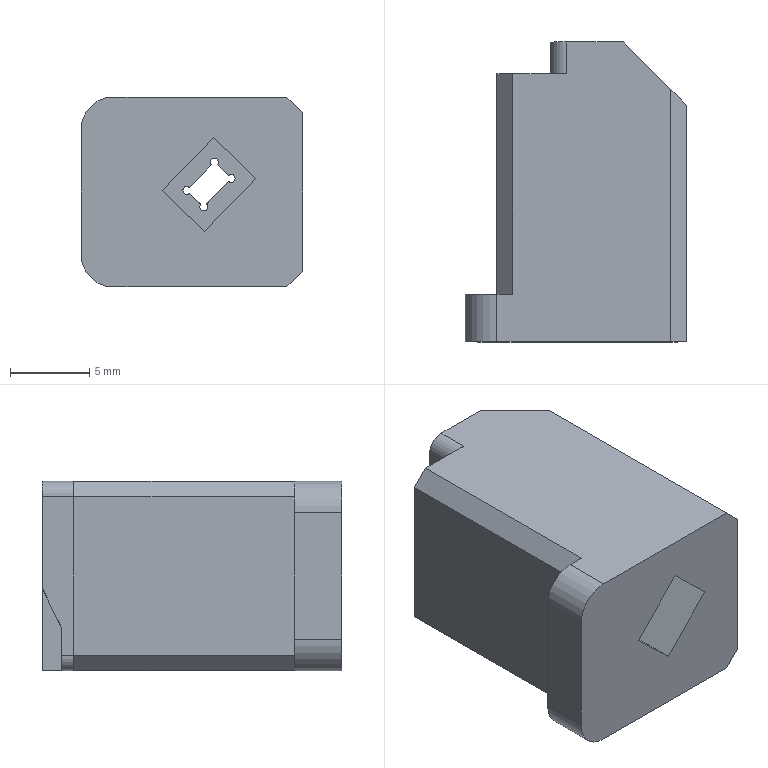Part | STEP file | 03-03 right cutter pad block | 1 solid | 46 faces | box 14 x 18.95 x 12 mm | volume 2331 mm3 | plane 29 | cylinder 17 | commonest cylinder face diameters 0.5 x9 0.6 x4 2 x2 4 x2
STEP:
#1=CARTESIAN_POINT('',(-2.2,16.95,-0.1351));
#2=VERTEX_POINT('',#1);
#3=CARTESIAN_POINT('',(-2.2,16.95,0.4649));
#4=VERTEX_POINT('',#3);
#5=CARTESIAN_POINT('',(-2.2,16.95,0.1649));
#6=DIRECTION('',(0.,1.,0.));
#7=DIRECTION('',(0.,0.,1.));
#8=AXIS2_PLACEMENT_3D('',#5,#6,#7);
#9=CIRCLE('',#8,0.3);
#10=EDGE_CURVE('',#2,#4,#9,.T.);
#11=ORIENTED_EDGE('',*,*,#10,.F.);
#12=CARTESIAN_POINT('',(-2.2,18.95,-0.1351));
#13=VERTEX_POINT('',#12);
#14=CARTESIAN_POINT('',(-2.2,16.95,-0.1351));
#15=DIRECTION('',(0.,1.,0.));
#16=VECTOR('',#15,1000.);
#17=LINE('',#14,#16);
#18=EDGE_CURVE('',#2,#13,#17,.T.);
#19=ORIENTED_EDGE('',*,*,#18,.T.);
#20=CARTESIAN_POINT('',(-2.2,18.95,0.4649));
#21=VERTEX_POINT('',#20);
#22=CARTESIAN_POINT('',(-2.2,18.95,0.1649));
#23=DIRECTION('',(0.,1.,0.));
#24=DIRECTION('',(0.,0.,1.));
#25=AXIS2_PLACEMENT_3D('',#22,#23,#24);
#26=CIRCLE('',#25,0.3);
#27=EDGE_CURVE('',#13,#21,#26,.T.);
#28=ORIENTED_EDGE('',*,*,#27,.T.);
#29=CARTESIAN_POINT('',(-2.2,16.95,0.4649));
#30=DIRECTION('',(0.,1.,0.));
#31=VECTOR('',#30,1000.);
#32=LINE('',#29,#31);
#33=EDGE_CURVE('',#4,#21,#32,.T.);
#34=ORIENTED_EDGE('',*,*,#33,.F.);
#35=EDGE_LOOP('',(#11,#19,#28,#34));
#36=FACE_OUTER_BOUND('',#35,.T.);
#37=CARTESIAN_POINT('',(-2.2,16.95,0.1649));
#38=DIRECTION('',(0.,1.,0.));
#39=DIRECTION('',(0.,0.,1.));
#40=AXIS2_PLACEMENT_3D('',#37,#38,#39);
#41=CYLINDRICAL_SURFACE('',#40,0.3);
#42=ADVANCED_FACE('',(#36),#41,.F.);
#43=CARTESIAN_POINT('',(-2.2,16.95,-1.435));
#44=VERTEX_POINT('',#43);
#45=CARTESIAN_POINT('',(-2.2,16.95,-0.8351));
#46=VERTEX_POINT('',#45);
#47=CARTESIAN_POINT('',(-2.2,16.95,-1.135));
#48=DIRECTION('',(0.,1.,0.));
#49=DIRECTION('',(0.,0.,1.));
#50=AXIS2_PLACEMENT_3D('',#47,#48,#49);
#51=CIRCLE('',#50,0.3);
#52=EDGE_CURVE('',#44,#46,#51,.T.);
#53=ORIENTED_EDGE('',*,*,#52,.F.);
#54=CARTESIAN_POINT('',(-2.2,18.619,-1.435));
#55=VERTEX_POINT('',#54);
#56=CARTESIAN_POINT('',(-2.2,16.95,-1.435));
#57=DIRECTION('',(0.,1.,0.));
#58=VECTOR('',#57,1000.);
#59=LINE('',#56,#58);
#60=EDGE_CURVE('',#44,#55,#59,.T.);
#61=ORIENTED_EDGE('',*,*,#60,.T.);
#62=CARTESIAN_POINT('',(-2.2,18.912,-0.8351));
#63=VERTEX_POINT('',#62);
#64=CARTESIAN_POINT('',(-2.2,18.912,-0.8351));
#65=CARTESIAN_POINT('',(-2.8,18.912,-0.8351));
#66=CARTESIAN_POINT('',(-2.8,18.619,-1.435));
#67=CARTESIAN_POINT('',(-2.2,18.619,-1.435));
#68=(BOUNDED_CURVE()B_SPLINE_CURVE(3,(#64,#65,#66,#67),.UNSPECIFIED.,.F.,.F.)B_SPLINE_CURVE_WITH_KNOTS((4,4),(0.,3.142),.UNSPECIFIED.)CURVE()GEOMETRIC_REPRESENTATION_ITEM()RATIONAL_B_SPLINE_CURVE((1.,0.3333,0.3333,1.))REPRESENTATION_ITEM(''));
#69=EDGE_CURVE('',#63,#55,#68,.T.);
#70=ORIENTED_EDGE('',*,*,#69,.F.);
#71=CARTESIAN_POINT('',(-2.2,16.95,-0.8351));
#72=DIRECTION('',(0.,1.,0.));
#73=VECTOR('',#72,1000.);
#74=LINE('',#71,#73);
#75=EDGE_CURVE('',#46,#63,#74,.T.);
#76=ORIENTED_EDGE('',*,*,#75,.F.);
#77=EDGE_LOOP('',(#53,#61,#70,#76));
#78=FACE_OUTER_BOUND('',#77,.T.);
#79=CARTESIAN_POINT('',(-2.2,16.95,-1.135));
#80=DIRECTION('',(0.,1.,0.));
#81=DIRECTION('',(0.,0.,1.));
#82=AXIS2_PLACEMENT_3D('',#79,#80,#81);
#83=CYLINDRICAL_SURFACE('',#82,0.3);
#84=ADVANCED_FACE('',(#78),#83,.F.);
#85=CARTESIAN_POINT('',(0.5868,12.,1.723));
#86=VERTEX_POINT('',#85);
#87=CARTESIAN_POINT('',(0.4071,12.,2.147));
#88=VERTEX_POINT('',#87);
#89=CARTESIAN_POINT('',(0.4071,12.,1.897));
#90=DIRECTION('',(0.,-1.,0.));
#91=DIRECTION('',(0.,0.,-1.));
#92=AXIS2_PLACEMENT_3D('',#89,#90,#91);
#93=CIRCLE('',#92,0.25);
#94=EDGE_CURVE('',#86,#88,#93,.T.);
#95=ORIENTED_EDGE('',*,*,#94,.T.);
#96=CARTESIAN_POINT('',(0.4071,18.95,2.147));
#97=VERTEX_POINT('',#96);
#98=CARTESIAN_POINT('',(0.4071,8.95,2.147));
#99=DIRECTION('',(0.,1.,0.));
#100=VECTOR('',#99,1000.);
#101=LINE('',#98,#100);
#102=EDGE_CURVE('',#88,#97,#101,.T.);
#103=ORIENTED_EDGE('',*,*,#102,.T.);
#104=CARTESIAN_POINT('',(0.5868,18.95,1.723));
#105=VERTEX_POINT('',#104);
#106=CARTESIAN_POINT('',(0.4071,18.95,1.897));
#107=DIRECTION('',(0.,1.,0.));
#108=DIRECTION('',(0.,0.,1.));
#109=AXIS2_PLACEMENT_3D('',#106,#107,#108);
#110=CIRCLE('',#109,0.25);
#111=EDGE_CURVE('',#97,#105,#110,.T.);
#112=ORIENTED_EDGE('',*,*,#111,.T.);
#113=CARTESIAN_POINT('',(0.5868,8.95,1.723));
#114=DIRECTION('',(0.,1.,0.));
#115=VECTOR('',#114,1000.);
#116=LINE('',#113,#115);
#117=EDGE_CURVE('',#86,#105,#116,.T.);
#118=ORIENTED_EDGE('',*,*,#117,.F.);
#119=EDGE_LOOP('',(#95,#103,#112,#118));
#120=FACE_OUTER_BOUND('',#119,.T.);
#121=CARTESIAN_POINT('',(0.4071,8.95,1.897));
#122=DIRECTION('',(0.,1.,0.));
#123=DIRECTION('',(0.,0.,1.));
#124=AXIS2_PLACEMENT_3D('',#121,#122,#123);
#125=CYLINDRICAL_SURFACE('',#124,0.25);
#126=ADVANCED_FACE('',(#120),#125,.F.);
#127=CARTESIAN_POINT('',(1.311,12.,0.6741));
#128=VERTEX_POINT('',#127);
#129=CARTESIAN_POINT('',(1.485,12.,0.6038));
#130=VERTEX_POINT('',#129);
#131=CARTESIAN_POINT('',(1.485,12.,0.8538));
#132=DIRECTION('',(0.,-1.,0.));
#133=DIRECTION('',(0.,0.,-1.));
#134=AXIS2_PLACEMENT_3D('',#131,#132,#133);
#135=CIRCLE('',#134,0.25);
#136=EDGE_CURVE('',#128,#130,#135,.T.);
#137=ORIENTED_EDGE('',*,*,#136,.T.);
#138=CARTESIAN_POINT('',(1.485,18.95,0.6038));
#139=VERTEX_POINT('',#138);
#140=CARTESIAN_POINT('',(1.485,8.95,0.6038));
#141=DIRECTION('',(0.,1.,0.));
#142=VECTOR('',#141,1000.);
#143=LINE('',#140,#142);
#144=EDGE_CURVE('',#130,#139,#143,.T.);
#145=ORIENTED_EDGE('',*,*,#144,.T.);
#146=CARTESIAN_POINT('',(1.311,18.95,0.6741));
#147=VERTEX_POINT('',#146);
#148=CARTESIAN_POINT('',(1.485,18.95,0.8538));
#149=DIRECTION('',(0.,1.,0.));
#150=DIRECTION('',(0.,0.,1.));
#151=AXIS2_PLACEMENT_3D('',#148,#149,#150);
#152=CIRCLE('',#151,0.25);
#153=EDGE_CURVE('',#139,#147,#152,.T.);
#154=ORIENTED_EDGE('',*,*,#153,.T.);
#155=CARTESIAN_POINT('',(1.311,8.95,0.6741));
#156=DIRECTION('',(0.,1.,0.));
#157=VECTOR('',#156,1000.);
#158=LINE('',#155,#157);
#159=EDGE_CURVE('',#128,#147,#158,.T.);
#160=ORIENTED_EDGE('',*,*,#159,.F.);
#161=EDGE_LOOP('',(#137,#145,#154,#160));
#162=FACE_OUTER_BOUND('',#161,.T.);
#163=CARTESIAN_POINT('',(1.485,8.95,0.8538));
#164=DIRECTION('',(0.,1.,0.));
#165=DIRECTION('',(0.,0.,1.));
#166=AXIS2_PLACEMENT_3D('',#163,#164,#165);
#167=CYLINDRICAL_SURFACE('',#166,0.25);
#168=ADVANCED_FACE('',(#162),#167,.F.);
#169=ORIENTED_EDGE('',*,*,#144,.F.);
#170=CARTESIAN_POINT('',(1.485,12.,1.104));
#171=VERTEX_POINT('',#170);
#172=CARTESIAN_POINT('',(1.485,12.,0.8538));
#173=DIRECTION('',(0.,-1.,0.));
#174=DIRECTION('',(0.,0.,-1.));
#175=AXIS2_PLACEMENT_3D('',#172,#173,#174);
#176=CIRCLE('',#175,0.25);
#177=EDGE_CURVE('',#130,#171,#176,.T.);
#178=ORIENTED_EDGE('',*,*,#177,.T.);
#179=CARTESIAN_POINT('',(1.485,18.95,1.104));
#180=VERTEX_POINT('',#179);
#181=CARTESIAN_POINT('',(1.485,8.95,1.104));
#182=DIRECTION('',(0.,1.,0.));
#183=VECTOR('',#182,1000.);
#184=LINE('',#181,#183);
#185=EDGE_CURVE('',#171,#180,#184,.T.);
#186=ORIENTED_EDGE('',*,*,#185,.T.);
#187=CARTESIAN_POINT('',(1.485,18.95,0.8538));
#188=DIRECTION('',(0.,1.,0.));
#189=DIRECTION('',(0.,0.,1.));
#190=AXIS2_PLACEMENT_3D('',#187,#188,#189);
#191=CIRCLE('',#190,0.25);
#192=EDGE_CURVE('',#180,#139,#191,.T.);
#193=ORIENTED_EDGE('',*,*,#192,.T.);
#194=EDGE_LOOP('',(#169,#178,#186,#193));
#195=FACE_OUTER_BOUND('',#194,.T.);
#196=CARTESIAN_POINT('',(1.485,8.95,0.8538));
#197=DIRECTION('',(0.,1.,0.));
#198=DIRECTION('',(0.,0.,1.));
#199=AXIS2_PLACEMENT_3D('',#196,#197,#198);
#200=CYLINDRICAL_SURFACE('',#199,0.25);
#201=ADVANCED_FACE('',(#195),#200,.F.);
#202=CARTESIAN_POINT('',(-1.331,12.,0.35));
#203=VERTEX_POINT('',#202);
#204=CARTESIAN_POINT('',(-1.331,12.,-0.15));
#205=VERTEX_POINT('',#204);
#206=CARTESIAN_POINT('',(-1.331,12.,0.1));
#207=DIRECTION('',(0.,-1.,0.));
#208=DIRECTION('',(0.,0.,-1.));
#209=AXIS2_PLACEMENT_3D('',#206,#207,#208);
#210=CIRCLE('',#209,0.25);
#211=EDGE_CURVE('',#203,#205,#210,.T.);
#212=ORIENTED_EDGE('',*,*,#211,.T.);
#213=CARTESIAN_POINT('',(-1.331,18.95,-0.15));
#214=VERTEX_POINT('',#213);
#215=CARTESIAN_POINT('',(-1.331,8.95,-0.15));
#216=DIRECTION('',(0.,1.,0.));
#217=VECTOR('',#216,1000.);
#218=LINE('',#215,#217);
#219=EDGE_CURVE('',#205,#214,#218,.T.);
#220=ORIENTED_EDGE('',*,*,#219,.T.);
#221=CARTESIAN_POINT('',(-1.331,18.95,0.35));
#222=VERTEX_POINT('',#221);
#223=CARTESIAN_POINT('',(-1.331,18.95,0.1));
#224=DIRECTION('',(0.,1.,0.));
#225=DIRECTION('',(0.,0.,1.));
#226=AXIS2_PLACEMENT_3D('',#223,#224,#225);
#227=CIRCLE('',#226,0.25);
#228=EDGE_CURVE('',#214,#222,#227,.T.);
#229=ORIENTED_EDGE('',*,*,#228,.T.);
#230=CARTESIAN_POINT('',(-1.331,8.95,0.35));
#231=DIRECTION('',(0.,1.,0.));
#232=VECTOR('',#231,1000.);
#233=LINE('',#230,#232);
#234=EDGE_CURVE('',#203,#222,#233,.T.);
#235=ORIENTED_EDGE('',*,*,#234,.F.);
#236=EDGE_LOOP('',(#212,#220,#229,#235));
#237=FACE_OUTER_BOUND('',#236,.T.);
#238=CARTESIAN_POINT('',(-1.331,8.95,0.1));
#239=DIRECTION('',(0.,1.,0.));
#240=DIRECTION('',(0.,0.,1.));
#241=AXIS2_PLACEMENT_3D('',#238,#239,#240);
#242=CYLINDRICAL_SURFACE('',#241,0.25);
#243=ADVANCED_FACE('',(#237),#242,.F.);
#244=CARTESIAN_POINT('',(-1.157,12.,0.2797));
#245=VERTEX_POINT('',#244);
#246=CARTESIAN_POINT('',(-1.331,12.,0.1));
#247=DIRECTION('',(0.,-1.,0.));
#248=DIRECTION('',(0.,0.,-1.));
#249=AXIS2_PLACEMENT_3D('',#246,#247,#248);
#250=CIRCLE('',#249,0.25);
#251=EDGE_CURVE('',#245,#203,#250,.T.);
#252=ORIENTED_EDGE('',*,*,#251,.T.);
#253=ORIENTED_EDGE('',*,*,#234,.T.);
#254=CARTESIAN_POINT('',(-1.157,18.95,0.2797));
#255=VERTEX_POINT('',#254);
#256=CARTESIAN_POINT('',(-1.331,18.95,0.1));
#257=DIRECTION('',(0.,1.,0.));
#258=DIRECTION('',(0.,0.,1.));
#259=AXIS2_PLACEMENT_3D('',#256,#257,#258);
#260=CIRCLE('',#259,0.25);
#261=EDGE_CURVE('',#222,#255,#260,.T.);
#262=ORIENTED_EDGE('',*,*,#261,.T.);
#263=CARTESIAN_POINT('',(-1.157,8.95,0.2797));
#264=DIRECTION('',(0.,1.,0.));
#265=VECTOR('',#264,1000.);
#266=LINE('',#263,#265);
#267=EDGE_CURVE('',#245,#255,#266,.T.);
#268=ORIENTED_EDGE('',*,*,#267,.F.);
#269=EDGE_LOOP('',(#252,#253,#262,#268));
#270=FACE_OUTER_BOUND('',#269,.T.);
#271=CARTESIAN_POINT('',(-1.331,8.95,0.1));
#272=DIRECTION('',(0.,1.,0.));
#273=DIRECTION('',(0.,0.,1.));
#274=AXIS2_PLACEMENT_3D('',#271,#272,#273);
#275=CYLINDRICAL_SURFACE('',#274,0.25);
#276=ADVANCED_FACE('',(#270),#275,.F.);
#277=CARTESIAN_POINT('',(1.305,12.,1.028));
#278=VERTEX_POINT('',#277);
#279=CARTESIAN_POINT('',(1.485,12.,0.8538));
#280=DIRECTION('',(0.7187,0.,-0.6953));
#281=VECTOR('',#280,1000.);
#282=LINE('',#279,#281);
#283=EDGE_CURVE('',#86,#278,#282,.T.);
#284=ORIENTED_EDGE('',*,*,#283,.F.);
#285=ORIENTED_EDGE('',*,*,#117,.T.);
#286=CARTESIAN_POINT('',(1.305,18.95,1.028));
#287=VERTEX_POINT('',#286);
#288=CARTESIAN_POINT('',(1.485,18.95,0.8538));
#289=DIRECTION('',(0.7187,0.,-0.6953));
#290=VECTOR('',#289,1000.);
#291=LINE('',#288,#290);
#292=EDGE_CURVE('',#105,#287,#291,.T.);
#293=ORIENTED_EDGE('',*,*,#292,.T.);
#294=CARTESIAN_POINT('',(1.305,8.95,1.028));
#295=DIRECTION('',(0.,-1.,0.));
#296=VECTOR('',#295,1000.);
#297=LINE('',#294,#296);
#298=EDGE_CURVE('',#287,#278,#297,.T.);
#299=ORIENTED_EDGE('',*,*,#298,.T.);
#300=EDGE_LOOP('',(#284,#285,#293,#299));
#301=FACE_OUTER_BOUND('',#300,.T.);
#302=CARTESIAN_POINT('',(1.485,-11.05,0.8538));
#303=DIRECTION('',(0.6953,0.,0.7187));
#304=DIRECTION('',(0.7187,0.,-0.6953));
#305=AXIS2_PLACEMENT_3D('',#302,#303,#304);
#306=PLANE('',#305);
#307=ADVANCED_FACE('',(#301),#306,.F.);
#308=CARTESIAN_POINT('',(0.2333,18.95,1.717));
#309=VERTEX_POINT('',#308);
#310=CARTESIAN_POINT('',(-1.331,18.95,0.1));
#311=DIRECTION('',(0.6953,0.,0.7187));
#312=VECTOR('',#311,1000.);
#313=LINE('',#310,#312);
#314=EDGE_CURVE('',#255,#309,#313,.T.);
#315=ORIENTED_EDGE('',*,*,#314,.T.);
#316=CARTESIAN_POINT('',(0.2333,12.,1.717));
#317=VERTEX_POINT('',#316);
#318=CARTESIAN_POINT('',(0.2333,8.95,1.717));
#319=DIRECTION('',(0.,-1.,0.));
#320=VECTOR('',#319,1000.);
#321=LINE('',#318,#320);
#322=EDGE_CURVE('',#309,#317,#321,.T.);
#323=ORIENTED_EDGE('',*,*,#322,.T.);
#324=CARTESIAN_POINT('',(-1.331,12.,0.1));
#325=DIRECTION('',(0.6953,0.,0.7187));
#326=VECTOR('',#325,1000.);
#327=LINE('',#324,#326);
#328=EDGE_CURVE('',#245,#317,#327,.T.);
#329=ORIENTED_EDGE('',*,*,#328,.F.);
#330=ORIENTED_EDGE('',*,*,#267,.T.);
#331=EDGE_LOOP('',(#315,#323,#329,#330));
#332=FACE_OUTER_BOUND('',#331,.T.);
#333=CARTESIAN_POINT('',(-1.331,-11.05,0.1));
#334=DIRECTION('',(-0.7187,0.,0.6953));
#335=DIRECTION('',(0.6953,0.,0.7187));
#336=AXIS2_PLACEMENT_3D('',#333,#334,#335);
#337=PLANE('',#336);
#338=ADVANCED_FACE('',(#332),#337,.F.);
#339=CARTESIAN_POINT('',(-0.0793,12.,-0.7633));
#340=VERTEX_POINT('',#339);
#341=CARTESIAN_POINT('',(-0.2531,12.,-0.943));
#342=DIRECTION('',(-0.6953,0.,-0.7187));
#343=VECTOR('',#342,1000.);
#344=LINE('',#341,#343);
#345=EDGE_CURVE('',#128,#340,#344,.T.);
#346=ORIENTED_EDGE('',*,*,#345,.F.);
#347=ORIENTED_EDGE('',*,*,#159,.T.);
#348=CARTESIAN_POINT('',(-0.07359,18.95,-0.7574));
#349=VERTEX_POINT('',#348);
#350=CARTESIAN_POINT('',(-0.2531,18.95,-0.943));
#351=DIRECTION('',(-0.6953,0.,-0.7187));
#352=VECTOR('',#351,1000.);
#353=LINE('',#350,#352);
#354=EDGE_CURVE('',#147,#349,#353,.T.);
#355=ORIENTED_EDGE('',*,*,#354,.T.);
#356=CARTESIAN_POINT('',(-0.0793,18.947,-0.7633));
#357=VERTEX_POINT('',#356);
#358=CARTESIAN_POINT('',(0.7208,19.35,0.06375));
#359=DIRECTION('',(0.6562,0.3308,0.6782));
#360=VECTOR('',#359,1000.);
#361=LINE('',#358,#360);
#362=EDGE_CURVE('',#357,#349,#361,.T.);
#363=ORIENTED_EDGE('',*,*,#362,.F.);
#364=CARTESIAN_POINT('',(-0.0793,8.95,-0.7633));
#365=DIRECTION('',(0.,-1.,0.));
#366=VECTOR('',#365,1000.);
#367=LINE('',#364,#366);
#368=EDGE_CURVE('',#357,#340,#367,.T.);
#369=ORIENTED_EDGE('',*,*,#368,.T.);
#370=EDGE_LOOP('',(#346,#347,#355,#363,#369));
#371=FACE_OUTER_BOUND('',#370,.T.);
#372=CARTESIAN_POINT('',(-0.2531,-11.05,-0.943));
#373=DIRECTION('',(0.7187,0.,-0.6953));
#374=DIRECTION('',(-0.6953,0.,-0.7187));
#375=AXIS2_PLACEMENT_3D('',#372,#373,#374);
#376=PLANE('',#375);
#377=ADVANCED_FACE('',(#371),#376,.F.);
#378=CARTESIAN_POINT('',(-0.4328,12.,-0.7691));
#379=VERTEX_POINT('',#378);
#380=CARTESIAN_POINT('',(-1.152,12.,-0.07383));
#381=VERTEX_POINT('',#380);
#382=CARTESIAN_POINT('',(-0.2531,12.,-0.943));
#383=DIRECTION('',(-0.7187,0.,0.6953));
#384=VECTOR('',#383,1000.);
#385=LINE('',#382,#384);
#386=EDGE_CURVE('',#379,#381,#385,.T.);
#387=ORIENTED_EDGE('',*,*,#386,.F.);
#388=CARTESIAN_POINT('',(-0.4328,18.944,-0.7691));
#389=VERTEX_POINT('',#388);
#390=CARTESIAN_POINT('',(-0.4328,8.95,-0.7691));
#391=DIRECTION('',(0.,1.,0.));
#392=VECTOR('',#391,1000.);
#393=LINE('',#390,#392);
#394=EDGE_CURVE('',#379,#389,#393,.T.);
#395=ORIENTED_EDGE('',*,*,#394,.T.);
#396=CARTESIAN_POINT('',(-0.4449,18.95,-0.7574));
#397=VERTEX_POINT('',#396);
#398=CARTESIAN_POINT('',(-0.1997,18.834,-0.9946));
#399=DIRECTION('',(0.6806,-0.3212,-0.6585));
#400=VECTOR('',#399,1000.);
#401=LINE('',#398,#400);
#402=EDGE_CURVE('',#397,#389,#401,.T.);
#403=ORIENTED_EDGE('',*,*,#402,.F.);
#404=CARTESIAN_POINT('',(-1.152,18.95,-0.07383));
#405=VERTEX_POINT('',#404);
#406=CARTESIAN_POINT('',(-0.2531,18.95,-0.943));
#407=DIRECTION('',(-0.7187,0.,0.6953));
#408=VECTOR('',#407,1000.);
#409=LINE('',#406,#408);
#410=EDGE_CURVE('',#397,#405,#409,.T.);
#411=ORIENTED_EDGE('',*,*,#410,.T.);
#412=CARTESIAN_POINT('',(-1.152,8.95,-0.07383));
#413=DIRECTION('',(0.,-1.,0.));
#414=VECTOR('',#413,1000.);
#415=LINE('',#412,#414);
#416=EDGE_CURVE('',#405,#381,#415,.T.);
#417=ORIENTED_EDGE('',*,*,#416,.T.);
#418=EDGE_LOOP('',(#387,#395,#403,#411,#417));
#419=FACE_OUTER_BOUND('',#418,.T.);
#420=CARTESIAN_POINT('',(-0.2531,-11.05,-0.943));
#421=DIRECTION('',(-0.6953,0.,-0.7187));
#422=DIRECTION('',(-0.7187,0.,0.6953));
#423=AXIS2_PLACEMENT_3D('',#420,#421,#422);
#424=PLANE('',#423);
#425=ADVANCED_FACE('',(#419),#424,.F.);
#426=CARTESIAN_POINT('',(-6.,16.95,-5.));
#427=VERTEX_POINT('',#426);
#428=CARTESIAN_POINT('',(-6.,3.,-5.));
#429=VERTEX_POINT('',#428);
#430=CARTESIAN_POINT('',(-6.,18.95,-5.));
#431=DIRECTION('',(0.,-1.,0.));
#432=VECTOR('',#431,1000.);
#433=LINE('',#430,#432);
#434=EDGE_CURVE('',#427,#429,#433,.T.);
#435=ORIENTED_EDGE('',*,*,#434,.T.);
#436=CARTESIAN_POINT('',(-6.,3.,5.));
#437=VERTEX_POINT('',#436);
#438=CARTESIAN_POINT('',(-6.,3.,-6.));
#439=DIRECTION('',(0.,0.,1.));
#440=VECTOR('',#439,1000.);
#441=LINE('',#438,#440);
#442=EDGE_CURVE('',#429,#437,#441,.T.);
#443=ORIENTED_EDGE('',*,*,#442,.T.);
#444=CARTESIAN_POINT('',(-6.,16.95,5.));
#445=VERTEX_POINT('',#444);
#446=CARTESIAN_POINT('',(-6.,18.95,5.));
#447=DIRECTION('',(0.,1.,0.));
#448=VECTOR('',#447,1000.);
#449=LINE('',#446,#448);
#450=EDGE_CURVE('',#437,#445,#449,.T.);
#451=ORIENTED_EDGE('',*,*,#450,.T.);
#452=CARTESIAN_POINT('',(-6.,16.95,-6.));
#453=DIRECTION('',(0.,0.,1.));
#454=VECTOR('',#453,1000.);
#455=LINE('',#452,#454);
#456=EDGE_CURVE('',#427,#445,#455,.T.);
#457=ORIENTED_EDGE('',*,*,#456,.F.);
#458=EDGE_LOOP('',(#435,#443,#451,#457));
#459=FACE_OUTER_BOUND('',#458,.T.);
#460=CARTESIAN_POINT('',(-6.,18.95,-6.));
#461=DIRECTION('',(1.,0.,0.));
#462=DIRECTION('',(0.,0.,-1.));
#463=AXIS2_PLACEMENT_3D('',#460,#461,#462);
#464=PLANE('',#463);
#465=ADVANCED_FACE('',(#459),#464,.F.);
#466=CARTESIAN_POINT('',(-5.,3.,-6.));
#467=VERTEX_POINT('',#466);
#468=CARTESIAN_POINT('',(-6.,3.,-5.));
#469=DIRECTION('',(0.7071,0.,-0.7071));
#470=VECTOR('',#469,1000.);
#471=LINE('',#468,#470);
#472=EDGE_CURVE('',#429,#467,#471,.T.);
#473=ORIENTED_EDGE('',*,*,#472,.F.);
#474=ORIENTED_EDGE('',*,*,#434,.F.);
#475=CARTESIAN_POINT('',(-5.,16.95,-6.));
#476=VERTEX_POINT('',#475);
#477=CARTESIAN_POINT('',(-6.,16.95,-5.));
#478=DIRECTION('',(0.7071,0.,-0.7071));
#479=VECTOR('',#478,1000.);
#480=LINE('',#477,#479);
#481=EDGE_CURVE('',#427,#476,#480,.T.);
#482=ORIENTED_EDGE('',*,*,#481,.T.);
#483=CARTESIAN_POINT('',(-5.,18.95,-6.));
#484=DIRECTION('',(0.,1.,0.));
#485=VECTOR('',#484,1000.);
#486=LINE('',#483,#485);
#487=EDGE_CURVE('',#467,#476,#486,.T.);
#488=ORIENTED_EDGE('',*,*,#487,.F.);
#489=EDGE_LOOP('',(#473,#474,#482,#488));
#490=FACE_OUTER_BOUND('',#489,.T.);
#491=CARTESIAN_POINT('',(-6.,18.95,-5.));
#492=DIRECTION('',(0.7071,0.,0.7071));
#493=DIRECTION('',(0.7071,0.,-0.7071));
#494=AXIS2_PLACEMENT_3D('',#491,#492,#493);
#495=PLANE('',#494);
#496=ADVANCED_FACE('',(#490),#495,.F.);
#497=CARTESIAN_POINT('',(-5.,3.,6.));
#498=VERTEX_POINT('',#497);
#499=CARTESIAN_POINT('',(-5.,3.,6.));
#500=DIRECTION('',(-0.7071,0.,-0.7071));
#501=VECTOR('',#500,1000.);
#502=LINE('',#499,#501);
#503=EDGE_CURVE('',#498,#437,#502,.T.);
#504=ORIENTED_EDGE('',*,*,#503,.F.);
#505=CARTESIAN_POINT('',(-5.,16.95,6.));
#506=VERTEX_POINT('',#505);
#507=CARTESIAN_POINT('',(-5.,18.95,6.));
#508=DIRECTION('',(0.,-1.,0.));
#509=VECTOR('',#508,1000.);
#510=LINE('',#507,#509);
#511=EDGE_CURVE('',#506,#498,#510,.T.);
#512=ORIENTED_EDGE('',*,*,#511,.F.);
#513=CARTESIAN_POINT('',(-5.,16.95,6.));
#514=DIRECTION('',(-0.7071,0.,-0.7071));
#515=VECTOR('',#514,1000.);
#516=LINE('',#513,#515);
#517=EDGE_CURVE('',#506,#445,#516,.T.);
#518=ORIENTED_EDGE('',*,*,#517,.T.);
#519=ORIENTED_EDGE('',*,*,#450,.F.);
#520=EDGE_LOOP('',(#504,#512,#518,#519));
#521=FACE_OUTER_BOUND('',#520,.T.);
#522=CARTESIAN_POINT('',(-5.,18.95,6.));
#523=DIRECTION('',(0.7071,0.,-0.7071));
#524=DIRECTION('',(-0.7071,0.,-0.7071));
#525=AXIS2_PLACEMENT_3D('',#522,#523,#524);
#526=PLANE('',#525);
#527=ADVANCED_FACE('',(#521),#526,.F.);
#528=CARTESIAN_POINT('',(6.,0.,-5.));
#529=VERTEX_POINT('',#528);
#530=CARTESIAN_POINT('',(6.,14.95,-5.));
#531=VERTEX_POINT('',#530);
#532=CARTESIAN_POINT('',(6.,18.95,-5.));
#533=DIRECTION('',(0.,1.,0.));
#534=VECTOR('',#533,1000.);
#535=LINE('',#532,#534);
#536=EDGE_CURVE('',#529,#531,#535,.T.);
#537=ORIENTED_EDGE('',*,*,#536,.T.);
#538=CARTESIAN_POINT('',(6.,14.95,5.));
#539=VERTEX_POINT('',#538);
#540=CARTESIAN_POINT('',(6.,14.95,5.));
#541=DIRECTION('',(0.,0.,1.));
#542=VECTOR('',#541,1000.);
#543=LINE('',#540,#542);
#544=EDGE_CURVE('',#531,#539,#543,.T.);
#545=ORIENTED_EDGE('',*,*,#544,.T.);
#546=CARTESIAN_POINT('',(6.,0.,5.));
#547=VERTEX_POINT('',#546);
#548=CARTESIAN_POINT('',(6.,18.95,5.));
#549=DIRECTION('',(0.,-1.,0.));
#550=VECTOR('',#549,1000.);
#551=LINE('',#548,#550);
#552=EDGE_CURVE('',#539,#547,#551,.T.);
#553=ORIENTED_EDGE('',*,*,#552,.T.);
#554=CARTESIAN_POINT('',(6.,0.,-6.));
#555=DIRECTION('',(0.,0.,-1.));
#556=VECTOR('',#555,1000.);
#557=LINE('',#554,#556);
#558=EDGE_CURVE('',#547,#529,#557,.T.);
#559=ORIENTED_EDGE('',*,*,#558,.T.);
#560=EDGE_LOOP('',(#537,#545,#553,#559));
#561=FACE_OUTER_BOUND('',#560,.T.);
#562=CARTESIAN_POINT('',(6.,18.95,-6.));
#563=DIRECTION('',(-1.,0.,0.));
#564=DIRECTION('',(0.,0.,1.));
#565=AXIS2_PLACEMENT_3D('',#562,#563,#564);
#566=PLANE('',#565);
#567=ADVANCED_FACE('',(#561),#566,.F.);
#568=CARTESIAN_POINT('',(5.,0.,-6.));
#569=VERTEX_POINT('',#568);
#570=CARTESIAN_POINT('',(-6.,0.,-6.));
#571=VERTEX_POINT('',#570);
#572=CARTESIAN_POINT('',(-6.,0.,-6.));
#573=DIRECTION('',(-1.,0.,0.));
#574=VECTOR('',#573,1000.);
#575=LINE('',#572,#574);
#576=EDGE_CURVE('',#569,#571,#575,.T.);
#577=ORIENTED_EDGE('',*,*,#576,.T.);
#578=CARTESIAN_POINT('',(-6.,3.,-6.));
#579=VERTEX_POINT('',#578);
#580=CARTESIAN_POINT('',(-6.,3.,-6.));
#581=DIRECTION('',(0.,1.,0.));
#582=VECTOR('',#581,1000.);
#583=LINE('',#580,#582);
#584=EDGE_CURVE('',#571,#579,#583,.T.);
#585=ORIENTED_EDGE('',*,*,#584,.T.);
#586=CARTESIAN_POINT('',(-5.,3.,-6.));
#587=DIRECTION('',(1.,0.,0.));
#588=VECTOR('',#587,1000.);
#589=LINE('',#586,#588);
#590=EDGE_CURVE('',#579,#467,#589,.T.);
#591=ORIENTED_EDGE('',*,*,#590,.T.);
#592=ORIENTED_EDGE('',*,*,#487,.T.);
#593=CARTESIAN_POINT('',(-1.6,16.95,-6.));
#594=VERTEX_POINT('',#593);
#595=CARTESIAN_POINT('',(-6.,16.95,-6.));
#596=DIRECTION('',(-1.,0.,0.));
#597=VECTOR('',#596,1000.);
#598=LINE('',#595,#597);
#599=EDGE_CURVE('',#594,#476,#598,.T.);
#600=ORIENTED_EDGE('',*,*,#599,.F.);
#601=CARTESIAN_POINT('',(-1.6,17.714,-6.));
#602=VERTEX_POINT('',#601);
#603=CARTESIAN_POINT('',(-1.6,18.95,-6.));
#604=DIRECTION('',(0.,1.,0.));
#605=VECTOR('',#604,1000.);
#606=LINE('',#603,#605);
#607=EDGE_CURVE('',#594,#602,#606,.T.);
#608=ORIENTED_EDGE('',*,*,#607,.T.);
#609=CARTESIAN_POINT('',(0.9,17.714,-6.));
#610=VERTEX_POINT('',#609);
#611=CARTESIAN_POINT('',(-6.,17.714,-6.));
#612=DIRECTION('',(1.,0.,0.));
#613=VECTOR('',#612,1000.);
#614=LINE('',#611,#613);
#615=EDGE_CURVE('',#602,#610,#614,.T.);
#616=ORIENTED_EDGE('',*,*,#615,.T.);
#617=CARTESIAN_POINT('',(0.9,18.95,-6.));
#618=VERTEX_POINT('',#617);
#619=CARTESIAN_POINT('',(0.9,18.95,-6.));
#620=DIRECTION('',(0.,1.,0.));
#621=VECTOR('',#620,1000.);
#622=LINE('',#619,#621);
#623=EDGE_CURVE('',#610,#618,#622,.T.);
#624=ORIENTED_EDGE('',*,*,#623,.T.);
#625=CARTESIAN_POINT('',(2.,18.95,-6.));
#626=VERTEX_POINT('',#625);
#627=CARTESIAN_POINT('',(-6.,18.95,-6.));
#628=DIRECTION('',(-1.,0.,0.));
#629=VECTOR('',#628,1000.);
#630=LINE('',#627,#629);
#631=EDGE_CURVE('',#626,#618,#630,.T.);
#632=ORIENTED_EDGE('',*,*,#631,.F.);
#633=CARTESIAN_POINT('',(5.,15.95,-6.));
#634=VERTEX_POINT('',#633);
#635=CARTESIAN_POINT('',(2.,18.95,-6.));
#636=DIRECTION('',(0.7071,-0.7071,0.));
#637=VECTOR('',#636,1000.);
#638=LINE('',#635,#637);
#639=EDGE_CURVE('',#626,#634,#638,.T.);
#640=ORIENTED_EDGE('',*,*,#639,.T.);
#641=CARTESIAN_POINT('',(5.,18.95,-6.));
#642=DIRECTION('',(0.,-1.,0.));
#643=VECTOR('',#642,1000.);
#644=LINE('',#641,#643);
#645=EDGE_CURVE('',#634,#569,#644,.T.);
#646=ORIENTED_EDGE('',*,*,#645,.T.);
#647=EDGE_LOOP('',(#577,#585,#591,#592,#600,#608,#616,#624,#632,#640,#646));
#648=FACE_OUTER_BOUND('',#647,.T.);
#649=CARTESIAN_POINT('',(-6.,18.95,-6.));
#650=DIRECTION('',(0.,0.,1.));
#651=DIRECTION('',(1.,0.,0.));
#652=AXIS2_PLACEMENT_3D('',#649,#650,#651);
#653=PLANE('',#652);
#654=ADVANCED_FACE('',(#648),#653,.F.);
#655=CARTESIAN_POINT('',(-6.,3.,6.));
#656=VERTEX_POINT('',#655);
#657=CARTESIAN_POINT('',(-5.,3.,6.));
#658=DIRECTION('',(-1.,0.,0.));
#659=VECTOR('',#658,1000.);
#660=LINE('',#657,#659);
#661=EDGE_CURVE('',#498,#656,#660,.T.);
#662=ORIENTED_EDGE('',*,*,#661,.T.);
#663=CARTESIAN_POINT('',(-6.,0.,6.));
#664=VERTEX_POINT('',#663);
#665=CARTESIAN_POINT('',(-6.,0.,6.));
#666=DIRECTION('',(0.,-1.,0.));
#667=VECTOR('',#666,1000.);
#668=LINE('',#665,#667);
#669=EDGE_CURVE('',#656,#664,#668,.T.);
#670=ORIENTED_EDGE('',*,*,#669,.T.);
#671=CARTESIAN_POINT('',(5.,0.,6.));
#672=VERTEX_POINT('',#671);
#673=CARTESIAN_POINT('',(-6.,0.,6.));
#674=DIRECTION('',(1.,0.,0.));
#675=VECTOR('',#674,1000.);
#676=LINE('',#673,#675);
#677=EDGE_CURVE('',#664,#672,#676,.T.);
#678=ORIENTED_EDGE('',*,*,#677,.T.);
#679=CARTESIAN_POINT('',(5.,15.95,6.));
#680=VERTEX_POINT('',#679);
#681=CARTESIAN_POINT('',(5.,18.95,6.));
#682=DIRECTION('',(0.,1.,0.));
#683=VECTOR('',#682,1000.);
#684=LINE('',#681,#683);
#685=EDGE_CURVE('',#672,#680,#684,.T.);
#686=ORIENTED_EDGE('',*,*,#685,.T.);
#687=CARTESIAN_POINT('',(2.,18.95,6.));
#688=VERTEX_POINT('',#687);
#689=CARTESIAN_POINT('',(2.,18.95,6.));
#690=DIRECTION('',(-0.7071,0.7071,0.));
#691=VECTOR('',#690,1000.);
#692=LINE('',#689,#691);
#693=EDGE_CURVE('',#680,#688,#692,.T.);
#694=ORIENTED_EDGE('',*,*,#693,.T.);
#695=CARTESIAN_POINT('',(-1.6,18.95,6.));
#696=VERTEX_POINT('',#695);
#697=CARTESIAN_POINT('',(-6.,18.95,6.));
#698=DIRECTION('',(1.,0.,0.));
#699=VECTOR('',#698,1000.);
#700=LINE('',#697,#699);
#701=EDGE_CURVE('',#696,#688,#700,.T.);
#702=ORIENTED_EDGE('',*,*,#701,.F.);
#703=CARTESIAN_POINT('',(-1.6,16.95,6.));
#704=VERTEX_POINT('',#703);
#705=CARTESIAN_POINT('',(-1.6,18.95,6.));
#706=DIRECTION('',(0.,-1.,0.));
#707=VECTOR('',#706,1000.);
#708=LINE('',#705,#707);
#709=EDGE_CURVE('',#696,#704,#708,.T.);
#710=ORIENTED_EDGE('',*,*,#709,.T.);
#711=CARTESIAN_POINT('',(-6.,16.95,6.));
#712=DIRECTION('',(1.,0.,0.));
#713=VECTOR('',#712,1000.);
#714=LINE('',#711,#713);
#715=EDGE_CURVE('',#506,#704,#714,.T.);
#716=ORIENTED_EDGE('',*,*,#715,.F.);
#717=ORIENTED_EDGE('',*,*,#511,.T.);
#718=EDGE_LOOP('',(#662,#670,#678,#686,#694,#702,#710,#716,#717));
#719=FACE_OUTER_BOUND('',#718,.T.);
#720=CARTESIAN_POINT('',(-6.,18.95,6.));
#721=DIRECTION('',(0.,0.,-1.));
#722=DIRECTION('',(-1.,0.,0.));
#723=AXIS2_PLACEMENT_3D('',#720,#721,#722);
#724=PLANE('',#723);
#725=ADVANCED_FACE('',(#719),#724,.F.);
#726=CARTESIAN_POINT('',(-2.2,18.95,0.1649));
#727=DIRECTION('',(0.,1.,0.));
#728=DIRECTION('',(0.,0.,1.));
#729=AXIS2_PLACEMENT_3D('',#726,#727,#728);
#730=CIRCLE('',#729,0.3);
#731=EDGE_CURVE('',#21,#13,#730,.T.);
#732=ORIENTED_EDGE('',*,*,#731,.F.);
#733=ORIENTED_EDGE('',*,*,#27,.F.);
#734=EDGE_LOOP('',(#732,#733));
#735=FACE_BOUND('',#734,.T.);
#736=CARTESIAN_POINT('',(0.4071,18.95,1.897));
#737=DIRECTION('',(0.,1.,0.));
#738=DIRECTION('',(0.,0.,1.));
#739=AXIS2_PLACEMENT_3D('',#736,#737,#738);
#740=CIRCLE('',#739,0.25);
#741=EDGE_CURVE('',#309,#97,#740,.T.);
#742=ORIENTED_EDGE('',*,*,#741,.F.);
#743=ORIENTED_EDGE('',*,*,#314,.F.);
#744=ORIENTED_EDGE('',*,*,#261,.F.);
#745=ORIENTED_EDGE('',*,*,#228,.F.);
#746=CARTESIAN_POINT('',(-1.331,18.95,0.1));
#747=DIRECTION('',(0.,1.,0.));
#748=DIRECTION('',(0.,0.,1.));
#749=AXIS2_PLACEMENT_3D('',#746,#747,#748);
#750=CIRCLE('',#749,0.25);
#751=EDGE_CURVE('',#405,#214,#750,.T.);
#752=ORIENTED_EDGE('',*,*,#751,.F.);
#753=ORIENTED_EDGE('',*,*,#410,.F.);
#754=CARTESIAN_POINT('',(-2.6,18.95,-0.7574));
#755=VERTEX_POINT('',#754);
#756=CARTESIAN_POINT('',(6.,18.95,-0.7574));
#757=DIRECTION('',(1.,0.,0.));
#758=VECTOR('',#757,1000.);
#759=LINE('',#756,#758);
#760=EDGE_CURVE('',#755,#397,#759,.T.);
#761=ORIENTED_EDGE('',*,*,#760,.F.);
#762=CARTESIAN_POINT('',(-2.6,18.95,5.));
#763=VERTEX_POINT('',#762);
#764=CARTESIAN_POINT('',(-2.6,18.95,-6.909));
#765=DIRECTION('',(0.,0.,-1.));
#766=VECTOR('',#765,1000.);
#767=LINE('',#764,#766);
#768=EDGE_CURVE('',#763,#755,#767,.T.);
#769=ORIENTED_EDGE('',*,*,#768,.F.);
#770=CARTESIAN_POINT('',(-1.6,18.95,5.));
#771=DIRECTION('',(0.,1.,0.));
#772=DIRECTION('',(0.,0.,1.));
#773=AXIS2_PLACEMENT_3D('',#770,#771,#772);
#774=CIRCLE('',#773,1.);
#775=EDGE_CURVE('',#763,#696,#774,.T.);
#776=ORIENTED_EDGE('',*,*,#775,.T.);
#777=ORIENTED_EDGE('',*,*,#701,.T.);
#778=CARTESIAN_POINT('',(2.,18.95,-5.));
#779=DIRECTION('',(0.,0.,-1.));
#780=VECTOR('',#779,1000.);
#781=LINE('',#778,#780);
#782=EDGE_CURVE('',#688,#626,#781,.T.);
#783=ORIENTED_EDGE('',*,*,#782,.T.);
#784=ORIENTED_EDGE('',*,*,#631,.T.);
#785=CARTESIAN_POINT('',(0.9,18.95,-0.7574));
#786=VERTEX_POINT('',#785);
#787=CARTESIAN_POINT('',(0.9,18.95,6.));
#788=DIRECTION('',(0.,0.,-1.));
#789=VECTOR('',#788,1000.);
#790=LINE('',#787,#789);
#791=EDGE_CURVE('',#786,#618,#790,.T.);
#792=ORIENTED_EDGE('',*,*,#791,.F.);
#793=CARTESIAN_POINT('',(6.,18.95,-0.7574));
#794=DIRECTION('',(1.,0.,0.));
#795=VECTOR('',#794,1000.);
#796=LINE('',#793,#795);
#797=EDGE_CURVE('',#349,#786,#796,.T.);
#798=ORIENTED_EDGE('',*,*,#797,.F.);
#799=ORIENTED_EDGE('',*,*,#354,.F.);
#800=ORIENTED_EDGE('',*,*,#153,.F.);
#801=ORIENTED_EDGE('',*,*,#192,.F.);
#802=CARTESIAN_POINT('',(1.485,18.95,0.8538));
#803=DIRECTION('',(0.,1.,0.));
#804=DIRECTION('',(0.,0.,1.));
#805=AXIS2_PLACEMENT_3D('',#802,#803,#804);
#806=CIRCLE('',#805,0.25);
#807=EDGE_CURVE('',#287,#180,#806,.T.);
#808=ORIENTED_EDGE('',*,*,#807,.F.);
#809=ORIENTED_EDGE('',*,*,#292,.F.);
#810=ORIENTED_EDGE('',*,*,#111,.F.);
#811=EDGE_LOOP('',(#742,#743,#744,#745,#752,#753,#761,#769,#776,#777,#783,#784,#792,#798,#799,#800,#801,#808,#809,#810));
#812=FACE_OUTER_BOUND('',#811,.T.);
#813=CARTESIAN_POINT('',(6.,18.95,6.));
#814=DIRECTION('',(0.,1.,0.));
#815=DIRECTION('',(0.,0.,1.));
#816=AXIS2_PLACEMENT_3D('',#813,#814,#815);
#817=PLANE('',#816);
#818=ADVANCED_FACE('',(#735,#812),#817,.T.);
#819=CARTESIAN_POINT('',(3.041,0.,0.8795));
#820=VERTEX_POINT('',#819);
#821=CARTESIAN_POINT('',(0.3813,0.,3.452));
#822=VERTEX_POINT('',#821);
#823=CARTESIAN_POINT('',(0.3813,0.,3.452));
#824=DIRECTION('',(-0.7187,0.,0.6953));
#825=VECTOR('',#824,1000.);
#826=LINE('',#823,#825);
#827=EDGE_CURVE('',#820,#822,#826,.T.);
#828=ORIENTED_EDGE('',*,*,#827,.F.);
#829=CARTESIAN_POINT('',(-0.2274,0.,-2.498));
#830=VERTEX_POINT('',#829);
#831=CARTESIAN_POINT('',(3.041,0.,0.8795));
#832=DIRECTION('',(0.6953,0.,0.7187));
#833=VECTOR('',#832,1000.);
#834=LINE('',#831,#833);
#835=EDGE_CURVE('',#830,#820,#834,.T.);
#836=ORIENTED_EDGE('',*,*,#835,.F.);
#837=CARTESIAN_POINT('',(-2.887,0.,0.07426));
#838=VERTEX_POINT('',#837);
#839=CARTESIAN_POINT('',(-2.887,0.,0.07426));
#840=DIRECTION('',(0.7187,0.,-0.6953));
#841=VECTOR('',#840,1000.);
#842=LINE('',#839,#841);
#843=EDGE_CURVE('',#838,#830,#842,.T.);
#844=ORIENTED_EDGE('',*,*,#843,.F.);
#845=CARTESIAN_POINT('',(-2.887,0.,0.07426));
#846=DIRECTION('',(-0.6953,0.,-0.7187));
#847=VECTOR('',#846,1000.);
#848=LINE('',#845,#847);
#849=EDGE_CURVE('',#822,#838,#848,.T.);
#850=ORIENTED_EDGE('',*,*,#849,.F.);
#851=EDGE_LOOP('',(#828,#836,#844,#850));
#852=FACE_BOUND('',#851,.T.);
#853=CARTESIAN_POINT('',(-8.,0.,4.));
#854=VERTEX_POINT('',#853);
#855=CARTESIAN_POINT('',(-8.,0.,-4.));
#856=VERTEX_POINT('',#855);
#857=CARTESIAN_POINT('',(-8.,0.,6.));
#858=DIRECTION('',(0.,0.,-1.));
#859=VECTOR('',#858,1000.);
#860=LINE('',#857,#859);
#861=EDGE_CURVE('',#854,#856,#860,.T.);
#862=ORIENTED_EDGE('',*,*,#861,.T.);
#863=CARTESIAN_POINT('',(-6.,0.,-4.));
#864=DIRECTION('',(0.,-1.,0.));
#865=DIRECTION('',(0.,0.,1.));
#866=AXIS2_PLACEMENT_3D('',#863,#864,#865);
#867=CIRCLE('',#866,2.);
#868=EDGE_CURVE('',#856,#571,#867,.T.);
#869=ORIENTED_EDGE('',*,*,#868,.T.);
#870=ORIENTED_EDGE('',*,*,#576,.F.);
#871=CARTESIAN_POINT('',(5.,0.,-6.));
#872=DIRECTION('',(0.7071,0.,0.7071));
#873=VECTOR('',#872,1000.);
#874=LINE('',#871,#873);
#875=EDGE_CURVE('',#569,#529,#874,.T.);
#876=ORIENTED_EDGE('',*,*,#875,.T.);
#877=ORIENTED_EDGE('',*,*,#558,.F.);
#878=CARTESIAN_POINT('',(6.,0.,5.));
#879=DIRECTION('',(-0.7071,0.,0.7071));
#880=VECTOR('',#879,1000.);
#881=LINE('',#878,#880);
#882=EDGE_CURVE('',#547,#672,#881,.T.);
#883=ORIENTED_EDGE('',*,*,#882,.T.);
#884=ORIENTED_EDGE('',*,*,#677,.F.);
#885=CARTESIAN_POINT('',(-6.,0.,4.));
#886=DIRECTION('',(0.,-1.,0.));
#887=DIRECTION('',(0.,0.,1.));
#888=AXIS2_PLACEMENT_3D('',#885,#886,#887);
#889=CIRCLE('',#888,2.);
#890=EDGE_CURVE('',#664,#854,#889,.T.);
#891=ORIENTED_EDGE('',*,*,#890,.T.);
#892=EDGE_LOOP('',(#862,#869,#870,#876,#877,#883,#884,#891));
#893=FACE_OUTER_BOUND('',#892,.T.);
#894=CARTESIAN_POINT('',(6.,0.,6.));
#895=DIRECTION('',(0.,1.,0.));
#896=DIRECTION('',(0.,0.,1.));
#897=AXIS2_PLACEMENT_3D('',#894,#895,#896);
#898=PLANE('',#897);
#899=ADVANCED_FACE('',(#852,#893),#898,.F.);
#900=ORIENTED_EDGE('',*,*,#552,.F.);
#901=CARTESIAN_POINT('',(4.667,16.283,6.333));
#902=DIRECTION('',(-0.5774,0.5774,0.5774));
#903=VECTOR('',#902,1000.);
#904=LINE('',#901,#903);
#905=EDGE_CURVE('',#539,#680,#904,.T.);
#906=ORIENTED_EDGE('',*,*,#905,.T.);
#907=ORIENTED_EDGE('',*,*,#685,.F.);
#908=ORIENTED_EDGE('',*,*,#882,.F.);
#909=EDGE_LOOP('',(#900,#906,#907,#908));
#910=FACE_OUTER_BOUND('',#909,.T.);
#911=CARTESIAN_POINT('',(6.,18.95,5.));
#912=DIRECTION('',(-0.7071,0.,-0.7071));
#913=DIRECTION('',(-0.7071,0.,0.7071));
#914=AXIS2_PLACEMENT_3D('',#911,#912,#913);
#915=PLANE('',#914);
#916=ADVANCED_FACE('',(#910),#915,.F.);
#917=ORIENTED_EDGE('',*,*,#645,.F.);
#918=CARTESIAN_POINT('',(4.,16.95,-7.));
#919=DIRECTION('',(0.5774,-0.5774,0.5774));
#920=VECTOR('',#919,1000.);
#921=LINE('',#918,#920);
#922=EDGE_CURVE('',#634,#531,#921,.T.);
#923=ORIENTED_EDGE('',*,*,#922,.T.);
#924=ORIENTED_EDGE('',*,*,#536,.F.);
#925=ORIENTED_EDGE('',*,*,#875,.F.);
#926=EDGE_LOOP('',(#917,#923,#924,#925));
#927=FACE_OUTER_BOUND('',#926,.T.);
#928=CARTESIAN_POINT('',(5.,18.95,-6.));
#929=DIRECTION('',(-0.7071,0.,0.7071));
#930=DIRECTION('',(0.7071,0.,0.7071));
#931=AXIS2_PLACEMENT_3D('',#928,#929,#930);
#932=PLANE('',#931);
#933=ADVANCED_FACE('',(#927),#932,.F.);
#934=CARTESIAN_POINT('',(-2.6,17.714,-3.292));
#935=VERTEX_POINT('',#934);
#936=CARTESIAN_POINT('',(-2.6,19.282,-0.07629));
#937=DIRECTION('',(0.,0.4384,0.8988));
#938=VECTOR('',#937,1000.);
#939=LINE('',#936,#938);
#940=EDGE_CURVE('',#935,#755,#939,.T.);
#941=ORIENTED_EDGE('',*,*,#940,.F.);
#942=CARTESIAN_POINT('',(-2.6,17.714,-5.));
#943=VERTEX_POINT('',#942);
#944=CARTESIAN_POINT('',(-2.6,17.714,-3.292));
#945=DIRECTION('',(0.,0.,1.));
#946=VECTOR('',#945,1000.);
#947=LINE('',#944,#946);
#948=EDGE_CURVE('',#943,#935,#947,.T.);
#949=ORIENTED_EDGE('',*,*,#948,.F.);
#950=CARTESIAN_POINT('',(-2.6,16.95,-5.));
#951=VERTEX_POINT('',#950);
#952=CARTESIAN_POINT('',(-2.6,16.95,-5.));
#953=DIRECTION('',(0.,-1.,0.));
#954=VECTOR('',#953,1000.);
#955=LINE('',#952,#954);
#956=EDGE_CURVE('',#943,#951,#955,.T.);
#957=ORIENTED_EDGE('',*,*,#956,.T.);
#958=CARTESIAN_POINT('',(-2.6,16.95,5.));
#959=VERTEX_POINT('',#958);
#960=CARTESIAN_POINT('',(-2.6,16.95,-6.909));
#961=DIRECTION('',(0.,0.,-1.));
#962=VECTOR('',#961,1000.);
#963=LINE('',#960,#962);
#964=EDGE_CURVE('',#959,#951,#963,.T.);
#965=ORIENTED_EDGE('',*,*,#964,.F.);
#966=CARTESIAN_POINT('',(-2.6,16.95,5.));
#967=DIRECTION('',(0.,1.,0.));
#968=VECTOR('',#967,1000.);
#969=LINE('',#966,#968);
#970=EDGE_CURVE('',#959,#763,#969,.T.);
#971=ORIENTED_EDGE('',*,*,#970,.T.);
#972=ORIENTED_EDGE('',*,*,#768,.T.);
#973=EDGE_LOOP('',(#941,#949,#957,#965,#971,#972));
#974=FACE_OUTER_BOUND('',#973,.T.);
#975=CARTESIAN_POINT('',(-2.6,16.95,-6.909));
#976=DIRECTION('',(1.,0.,0.));
#977=DIRECTION('',(0.,0.,-1.));
#978=AXIS2_PLACEMENT_3D('',#975,#976,#977);
#979=PLANE('',#978);
#980=ADVANCED_FACE('',(#974),#979,.F.);
#981=ORIENTED_EDGE('',*,*,#599,.T.);
#982=ORIENTED_EDGE('',*,*,#481,.F.);
#983=ORIENTED_EDGE('',*,*,#456,.T.);
#984=ORIENTED_EDGE('',*,*,#517,.F.);
#985=ORIENTED_EDGE('',*,*,#715,.T.);
#986=CARTESIAN_POINT('',(-1.6,16.95,5.));
#987=DIRECTION('',(0.,-1.,0.));
#988=DIRECTION('',(0.,0.,1.));
#989=AXIS2_PLACEMENT_3D('',#986,#987,#988);
#990=CIRCLE('',#989,1.);
#991=EDGE_CURVE('',#704,#959,#990,.T.);
#992=ORIENTED_EDGE('',*,*,#991,.T.);
#993=ORIENTED_EDGE('',*,*,#964,.T.);
#994=CARTESIAN_POINT('',(-1.6,16.95,-5.));
#995=DIRECTION('',(0.,-1.,0.));
#996=DIRECTION('',(0.,0.,1.));
#997=AXIS2_PLACEMENT_3D('',#994,#995,#996);
#998=CIRCLE('',#997,1.);
#999=EDGE_CURVE('',#951,#594,#998,.T.);
#1000=ORIENTED_EDGE('',*,*,#999,.T.);
#1001=EDGE_LOOP('',(#981,#982,#983,#984,#985,#992,#993,#1000));
#1002=FACE_OUTER_BOUND('',#1001,.T.);
#1003=CARTESIAN_POINT('',(-6.849,16.95,6.372));
#1004=DIRECTION('',(0.,1.,0.));
#1005=DIRECTION('',(0.,0.,1.));
#1006=AXIS2_PLACEMENT_3D('',#1003,#1004,#1005);
#1007=PLANE('',#1006);
#1008=ADVANCED_FACE('',(#1002),#1007,.T.);
#1009=ORIENTED_EDGE('',*,*,#775,.F.);
#1010=ORIENTED_EDGE('',*,*,#970,.F.);
#1011=ORIENTED_EDGE('',*,*,#991,.F.);
#1012=ORIENTED_EDGE('',*,*,#709,.F.);
#1013=EDGE_LOOP('',(#1009,#1010,#1011,#1012));
#1014=FACE_OUTER_BOUND('',#1013,.T.);
#1015=CARTESIAN_POINT('',(-1.6,18.95,5.));
#1016=DIRECTION('',(0.,-1.,0.));
#1017=DIRECTION('',(0.,0.,-1.));
#1018=AXIS2_PLACEMENT_3D('',#1015,#1016,#1017);
#1019=CYLINDRICAL_SURFACE('',#1018,1.);
#1020=ADVANCED_FACE('',(#1014),#1019,.T.);
#1021=CARTESIAN_POINT('',(-1.6,17.714,-5.));
#1022=DIRECTION('',(0.,1.,0.));
#1023=DIRECTION('',(0.,0.,-1.));
#1024=AXIS2_PLACEMENT_3D('',#1021,#1022,#1023);
#1025=CIRCLE('',#1024,1.);
#1026=EDGE_CURVE('',#602,#943,#1025,.T.);
#1027=ORIENTED_EDGE('',*,*,#1026,.F.);
#1028=ORIENTED_EDGE('',*,*,#607,.F.);
#1029=ORIENTED_EDGE('',*,*,#999,.F.);
#1030=ORIENTED_EDGE('',*,*,#956,.F.);
#1031=EDGE_LOOP('',(#1027,#1028,#1029,#1030));
#1032=FACE_OUTER_BOUND('',#1031,.T.);
#1033=CARTESIAN_POINT('',(-1.6,18.95,-5.));
#1034=DIRECTION('',(0.,1.,0.));
#1035=DIRECTION('',(0.,0.,1.));
#1036=AXIS2_PLACEMENT_3D('',#1033,#1034,#1035);
#1037=CYLINDRICAL_SURFACE('',#1036,1.);
#1038=ADVANCED_FACE('',(#1032),#1037,.T.);
#1039=CARTESIAN_POINT('',(0.9,17.714,-3.292));
#1040=VERTEX_POINT('',#1039);
#1041=CARTESIAN_POINT('',(0.9,17.714,-3.292));
#1042=DIRECTION('',(0.,0.,1.));
#1043=VECTOR('',#1042,1000.);
#1044=LINE('',#1041,#1043);
#1045=EDGE_CURVE('',#610,#1040,#1044,.T.);
#1046=ORIENTED_EDGE('',*,*,#1045,.T.);
#1047=CARTESIAN_POINT('',(0.9,19.282,-0.07629));
#1048=DIRECTION('',(0.,0.4384,0.8988));
#1049=VECTOR('',#1048,1000.);
#1050=LINE('',#1047,#1049);
#1051=EDGE_CURVE('',#1040,#786,#1050,.T.);
#1052=ORIENTED_EDGE('',*,*,#1051,.T.);
#1053=ORIENTED_EDGE('',*,*,#791,.T.);
#1054=ORIENTED_EDGE('',*,*,#623,.F.);
#1055=EDGE_LOOP('',(#1046,#1052,#1053,#1054));
#1056=FACE_OUTER_BOUND('',#1055,.T.);
#1057=CARTESIAN_POINT('',(0.9,17.714,-6.209));
#1058=DIRECTION('',(1.,0.,0.));
#1059=DIRECTION('',(0.,0.,-1.));
#1060=AXIS2_PLACEMENT_3D('',#1057,#1058,#1059);
#1061=PLANE('',#1060);
#1062=ADVANCED_FACE('',(#1056),#1061,.F.);
#1063=ORIENTED_EDGE('',*,*,#1026,.T.);
#1064=ORIENTED_EDGE('',*,*,#948,.T.);
#1065=CARTESIAN_POINT('',(0.9,17.714,-3.292));
#1066=DIRECTION('',(-1.,0.,0.));
#1067=VECTOR('',#1066,1000.);
#1068=LINE('',#1065,#1067);
#1069=EDGE_CURVE('',#1040,#935,#1068,.T.);
#1070=ORIENTED_EDGE('',*,*,#1069,.F.);
#1071=ORIENTED_EDGE('',*,*,#1045,.F.);
#1072=ORIENTED_EDGE('',*,*,#615,.F.);
#1073=EDGE_LOOP('',(#1063,#1064,#1070,#1071,#1072));
#1074=FACE_OUTER_BOUND('',#1073,.T.);
#1075=CARTESIAN_POINT('',(0.9,17.714,-3.292));
#1076=DIRECTION('',(0.,-1.,0.));
#1077=DIRECTION('',(0.,0.,-1.));
#1078=AXIS2_PLACEMENT_3D('',#1075,#1076,#1077);
#1079=PLANE('',#1078);
#1080=ADVANCED_FACE('',(#1074),#1079,.F.);
#1081=ORIENTED_EDGE('',*,*,#69,.T.);
#1082=CARTESIAN_POINT('',(-2.2,18.619,-1.435));
#1083=CARTESIAN_POINT('',(-1.6,18.619,-1.435));
#1084=CARTESIAN_POINT('',(-1.6,18.912,-0.8351));
#1085=CARTESIAN_POINT('',(-2.2,18.912,-0.8351));
#1086=(BOUNDED_CURVE()B_SPLINE_CURVE(3,(#1082,#1083,#1084,#1085),.UNSPECIFIED.,.F.,.F.)B_SPLINE_CURVE_WITH_KNOTS((4,4),(3.142,6.283),.UNSPECIFIED.)CURVE()GEOMETRIC_REPRESENTATION_ITEM()RATIONAL_B_SPLINE_CURVE((1.,0.3333,0.3333,1.))REPRESENTATION_ITEM(''));
#1087=EDGE_CURVE('',#55,#63,#1086,.T.);
#1088=ORIENTED_EDGE('',*,*,#1087,.T.);
#1089=EDGE_LOOP('',(#1081,#1088));
#1090=FACE_BOUND('',#1089,.T.);
#1091=ORIENTED_EDGE('',*,*,#402,.T.);
#1092=CARTESIAN_POINT('',(-0.4328,18.944,-0.7691));
#1093=CARTESIAN_POINT('',(-0.6147,18.853,-0.9572));
#1094=CARTESIAN_POINT('',(-0.5106,18.735,-1.197));
#1095=CARTESIAN_POINT('',(-0.249,18.738,-1.193));
#1096=CARTESIAN_POINT('',(0.01264,18.74,-1.189));
#1097=CARTESIAN_POINT('',(0.1088,18.858,-0.9452));
#1098=CARTESIAN_POINT('',(-0.0793,18.947,-0.7633));
#1099=(BOUNDED_CURVE()B_SPLINE_CURVE(3,(#1092,#1093,#1094,#1095,#1096,#1097,#1098),.UNSPECIFIED.,.F.,.F.)B_SPLINE_CURVE_WITH_KNOTS((4,3,4),(0.8019,3.158,5.514),.UNSPECIFIED.)CURVE()GEOMETRIC_REPRESENTATION_ITEM()RATIONAL_B_SPLINE_CURVE((1.,0.5885,0.5885,1.,0.5885,0.5885,1.))REPRESENTATION_ITEM(''));
#1100=EDGE_CURVE('',#389,#357,#1099,.T.);
#1101=ORIENTED_EDGE('',*,*,#1100,.T.);
#1102=ORIENTED_EDGE('',*,*,#362,.T.);
#1103=ORIENTED_EDGE('',*,*,#797,.T.);
#1104=ORIENTED_EDGE('',*,*,#1051,.F.);
#1105=ORIENTED_EDGE('',*,*,#1069,.T.);
#1106=ORIENTED_EDGE('',*,*,#940,.T.);
#1107=ORIENTED_EDGE('',*,*,#760,.T.);
#1108=EDGE_LOOP('',(#1091,#1101,#1102,#1103,#1104,#1105,#1106,#1107));
#1109=FACE_OUTER_BOUND('',#1108,.T.);
#1110=CARTESIAN_POINT('',(0.9,19.282,-0.07629));
#1111=DIRECTION('',(0.,-0.8988,0.4384));
#1112=DIRECTION('',(0.,-0.4384,-0.8988));
#1113=AXIS2_PLACEMENT_3D('',#1110,#1111,#1112);
#1114=PLANE('',#1113);
#1115=ADVANCED_FACE('',(#1090,#1109),#1114,.F.);
#1116=ORIENTED_EDGE('',*,*,#905,.F.);
#1117=ORIENTED_EDGE('',*,*,#544,.F.);
#1118=ORIENTED_EDGE('',*,*,#922,.F.);
#1119=ORIENTED_EDGE('',*,*,#639,.F.);
#1120=ORIENTED_EDGE('',*,*,#782,.F.);
#1121=ORIENTED_EDGE('',*,*,#693,.F.);
#1122=EDGE_LOOP('',(#1116,#1117,#1118,#1119,#1120,#1121));
#1123=FACE_OUTER_BOUND('',#1122,.T.);
#1124=CARTESIAN_POINT('',(2.,18.95,6.));
#1125=DIRECTION('',(0.7071,0.7071,0.));
#1126=DIRECTION('',(-0.7071,0.7071,0.));
#1127=AXIS2_PLACEMENT_3D('',#1124,#1125,#1126);
#1128=PLANE('',#1127);
#1129=ADVANCED_FACE('',(#1123),#1128,.T.);
#1130=CARTESIAN_POINT('',(-8.,3.,4.));
#1131=VERTEX_POINT('',#1130);
#1132=CARTESIAN_POINT('',(-8.,3.,-4.));
#1133=VERTEX_POINT('',#1132);
#1134=CARTESIAN_POINT('',(-8.,3.,6.));
#1135=DIRECTION('',(0.,0.,-1.));
#1136=VECTOR('',#1135,1000.);
#1137=LINE('',#1134,#1136);
#1138=EDGE_CURVE('',#1131,#1133,#1137,.T.);
#1139=ORIENTED_EDGE('',*,*,#1138,.T.);
#1140=CARTESIAN_POINT('',(-8.,0.,-4.));
#1141=DIRECTION('',(0.,-1.,0.));
#1142=VECTOR('',#1141,1000.);
#1143=LINE('',#1140,#1142);
#1144=EDGE_CURVE('',#1133,#856,#1143,.T.);
#1145=ORIENTED_EDGE('',*,*,#1144,.T.);
#1146=ORIENTED_EDGE('',*,*,#861,.F.);
#1147=CARTESIAN_POINT('',(-8.,3.,4.));
#1148=DIRECTION('',(0.,1.,0.));
#1149=VECTOR('',#1148,1000.);
#1150=LINE('',#1147,#1149);
#1151=EDGE_CURVE('',#854,#1131,#1150,.T.);
#1152=ORIENTED_EDGE('',*,*,#1151,.T.);
#1153=EDGE_LOOP('',(#1139,#1145,#1146,#1152));
#1154=FACE_OUTER_BOUND('',#1153,.T.);
#1155=CARTESIAN_POINT('',(-8.,3.,6.));
#1156=DIRECTION('',(-1.,0.,0.));
#1157=DIRECTION('',(0.,0.,1.));
#1158=AXIS2_PLACEMENT_3D('',#1155,#1156,#1157);
#1159=PLANE('',#1158);
#1160=ADVANCED_FACE('',(#1154),#1159,.T.);
#1161=ORIENTED_EDGE('',*,*,#590,.F.);
#1162=CARTESIAN_POINT('',(-6.,3.,-4.));
#1163=DIRECTION('',(0.,1.,0.));
#1164=DIRECTION('',(0.,0.,1.));
#1165=AXIS2_PLACEMENT_3D('',#1162,#1163,#1164);
#1166=CIRCLE('',#1165,2.);
#1167=EDGE_CURVE('',#579,#1133,#1166,.T.);
#1168=ORIENTED_EDGE('',*,*,#1167,.T.);
#1169=ORIENTED_EDGE('',*,*,#1138,.F.);
#1170=CARTESIAN_POINT('',(-6.,3.,4.));
#1171=DIRECTION('',(0.,1.,0.));
#1172=DIRECTION('',(0.,0.,1.));
#1173=AXIS2_PLACEMENT_3D('',#1170,#1171,#1172);
#1174=CIRCLE('',#1173,2.);
#1175=EDGE_CURVE('',#1131,#656,#1174,.T.);
#1176=ORIENTED_EDGE('',*,*,#1175,.T.);
#1177=ORIENTED_EDGE('',*,*,#661,.F.);
#1178=ORIENTED_EDGE('',*,*,#503,.T.);
#1179=ORIENTED_EDGE('',*,*,#442,.F.);
#1180=ORIENTED_EDGE('',*,*,#472,.T.);
#1181=EDGE_LOOP('',(#1161,#1168,#1169,#1176,#1177,#1178,#1179,#1180));
#1182=FACE_OUTER_BOUND('',#1181,.T.);
#1183=CARTESIAN_POINT('',(-5.,3.,-6.));
#1184=DIRECTION('',(0.,1.,0.));
#1185=DIRECTION('',(0.,0.,1.));
#1186=AXIS2_PLACEMENT_3D('',#1183,#1184,#1185);
#1187=PLANE('',#1186);
#1188=ADVANCED_FACE('',(#1182),#1187,.T.);
#1189=ORIENTED_EDGE('',*,*,#1167,.F.);
#1190=ORIENTED_EDGE('',*,*,#584,.F.);
#1191=ORIENTED_EDGE('',*,*,#868,.F.);
#1192=ORIENTED_EDGE('',*,*,#1144,.F.);
#1193=EDGE_LOOP('',(#1189,#1190,#1191,#1192));
#1194=FACE_OUTER_BOUND('',#1193,.T.);
#1195=CARTESIAN_POINT('',(-6.,3.,-4.));
#1196=DIRECTION('',(0.,1.,0.));
#1197=DIRECTION('',(0.,0.,1.));
#1198=AXIS2_PLACEMENT_3D('',#1195,#1196,#1197);
#1199=CYLINDRICAL_SURFACE('',#1198,2.);
#1200=ADVANCED_FACE('',(#1194),#1199,.T.);
#1201=ORIENTED_EDGE('',*,*,#1175,.F.);
#1202=ORIENTED_EDGE('',*,*,#1151,.F.);
#1203=ORIENTED_EDGE('',*,*,#890,.F.);
#1204=ORIENTED_EDGE('',*,*,#669,.F.);
#1205=EDGE_LOOP('',(#1201,#1202,#1203,#1204));
#1206=FACE_OUTER_BOUND('',#1205,.T.);
#1207=CARTESIAN_POINT('',(-6.,18.95,4.));
#1208=DIRECTION('',(0.,1.,0.));
#1209=DIRECTION('',(0.,0.,1.));
#1210=AXIS2_PLACEMENT_3D('',#1207,#1208,#1209);
#1211=CYLINDRICAL_SURFACE('',#1210,2.);
#1212=ADVANCED_FACE('',(#1206),#1211,.T.);
#1213=ORIENTED_EDGE('',*,*,#94,.F.);
#1214=ORIENTED_EDGE('',*,*,#283,.T.);
#1215=CARTESIAN_POINT('',(1.485,12.,0.8538));
#1216=DIRECTION('',(0.,-1.,0.));
#1217=DIRECTION('',(0.,0.,-1.));
#1218=AXIS2_PLACEMENT_3D('',#1215,#1216,#1217);
#1219=CIRCLE('',#1218,0.25);
#1220=EDGE_CURVE('',#171,#278,#1219,.T.);
#1221=ORIENTED_EDGE('',*,*,#1220,.F.);
#1222=ORIENTED_EDGE('',*,*,#177,.F.);
#1223=ORIENTED_EDGE('',*,*,#136,.F.);
#1224=ORIENTED_EDGE('',*,*,#345,.T.);
#1225=CARTESIAN_POINT('',(-0.2531,12.,-0.943));
#1226=DIRECTION('',(0.,-1.,0.));
#1227=DIRECTION('',(0.,0.,-1.));
#1228=AXIS2_PLACEMENT_3D('',#1225,#1226,#1227);
#1229=CIRCLE('',#1228,0.25);
#1230=EDGE_CURVE('',#379,#340,#1229,.T.);
#1231=ORIENTED_EDGE('',*,*,#1230,.F.);
#1232=ORIENTED_EDGE('',*,*,#386,.T.);
#1233=CARTESIAN_POINT('',(-1.331,12.,0.1));
#1234=DIRECTION('',(0.,-1.,0.));
#1235=DIRECTION('',(0.,0.,-1.));
#1236=AXIS2_PLACEMENT_3D('',#1233,#1234,#1235);
#1237=CIRCLE('',#1236,0.25);
#1238=EDGE_CURVE('',#205,#381,#1237,.T.);
#1239=ORIENTED_EDGE('',*,*,#1238,.F.);
#1240=ORIENTED_EDGE('',*,*,#211,.F.);
#1241=ORIENTED_EDGE('',*,*,#251,.F.);
#1242=ORIENTED_EDGE('',*,*,#328,.T.);
#1243=CARTESIAN_POINT('',(0.4071,12.,1.897));
#1244=DIRECTION('',(0.,-1.,0.));
#1245=DIRECTION('',(0.,0.,-1.));
#1246=AXIS2_PLACEMENT_3D('',#1243,#1244,#1245);
#1247=CIRCLE('',#1246,0.25);
#1248=EDGE_CURVE('',#88,#317,#1247,.T.);
#1249=ORIENTED_EDGE('',*,*,#1248,.F.);
#1250=EDGE_LOOP('',(#1213,#1214,#1221,#1222,#1223,#1224,#1231,#1232,#1239,#1240,#1241,#1242,#1249));
#1251=FACE_BOUND('',#1250,.T.);
#1252=CARTESIAN_POINT('',(-0.2274,12.,-2.498));
#1253=VERTEX_POINT('',#1252);
#1254=CARTESIAN_POINT('',(3.041,12.,0.8795));
#1255=VERTEX_POINT('',#1254);
#1256=CARTESIAN_POINT('',(3.041,12.,0.8795));
#1257=DIRECTION('',(0.6953,0.,0.7187));
#1258=VECTOR('',#1257,1000.);
#1259=LINE('',#1256,#1258);
#1260=EDGE_CURVE('',#1253,#1255,#1259,.T.);
#1261=ORIENTED_EDGE('',*,*,#1260,.T.);
#1262=CARTESIAN_POINT('',(0.3813,12.,3.452));
#1263=VERTEX_POINT('',#1262);
#1264=CARTESIAN_POINT('',(0.3813,12.,3.452));
#1265=DIRECTION('',(-0.7187,0.,0.6953));
#1266=VECTOR('',#1265,1000.);
#1267=LINE('',#1264,#1266);
#1268=EDGE_CURVE('',#1255,#1263,#1267,.T.);
#1269=ORIENTED_EDGE('',*,*,#1268,.T.);
#1270=CARTESIAN_POINT('',(-2.887,12.,0.07426));
#1271=VERTEX_POINT('',#1270);
#1272=CARTESIAN_POINT('',(-2.887,12.,0.07426));
#1273=DIRECTION('',(-0.6953,0.,-0.7187));
#1274=VECTOR('',#1273,1000.);
#1275=LINE('',#1272,#1274);
#1276=EDGE_CURVE('',#1263,#1271,#1275,.T.);
#1277=ORIENTED_EDGE('',*,*,#1276,.T.);
#1278=CARTESIAN_POINT('',(-2.887,12.,0.07426));
#1279=DIRECTION('',(0.7187,0.,-0.6953));
#1280=VECTOR('',#1279,1000.);
#1281=LINE('',#1278,#1280);
#1282=EDGE_CURVE('',#1271,#1253,#1281,.T.);
#1283=ORIENTED_EDGE('',*,*,#1282,.T.);
#1284=EDGE_LOOP('',(#1261,#1269,#1277,#1283));
#1285=FACE_OUTER_BOUND('',#1284,.T.);
#1286=CARTESIAN_POINT('',(-0.2274,12.,-2.498));
#1287=DIRECTION('',(0.,-1.,0.));
#1288=DIRECTION('',(0.,0.,-1.));
#1289=AXIS2_PLACEMENT_3D('',#1286,#1287,#1288);
#1290=PLANE('',#1289);
#1291=ADVANCED_FACE('',(#1251,#1285),#1290,.T.);
#1292=ORIENTED_EDGE('',*,*,#835,.T.);
#1293=CARTESIAN_POINT('',(3.041,12.,0.8795));
#1294=DIRECTION('',(0.,-1.,0.));
#1295=VECTOR('',#1294,1000.);
#1296=LINE('',#1293,#1295);
#1297=EDGE_CURVE('',#1255,#820,#1296,.T.);
#1298=ORIENTED_EDGE('',*,*,#1297,.F.);
#1299=ORIENTED_EDGE('',*,*,#1260,.F.);
#1300=CARTESIAN_POINT('',(-0.2274,12.,-2.498));
#1301=DIRECTION('',(0.,-1.,0.));
#1302=VECTOR('',#1301,1000.);
#1303=LINE('',#1300,#1302);
#1304=EDGE_CURVE('',#1253,#830,#1303,.T.);
#1305=ORIENTED_EDGE('',*,*,#1304,.T.);
#1306=EDGE_LOOP('',(#1292,#1298,#1299,#1305));
#1307=FACE_OUTER_BOUND('',#1306,.T.);
#1308=CARTESIAN_POINT('',(3.041,12.,0.8795));
#1309=DIRECTION('',(0.7187,0.,-0.6953));
#1310=DIRECTION('',(-0.6953,0.,-0.7187));
#1311=AXIS2_PLACEMENT_3D('',#1308,#1309,#1310);
#1312=PLANE('',#1311);
#1313=ADVANCED_FACE('',(#1307),#1312,.F.);
#1314=ORIENTED_EDGE('',*,*,#843,.T.);
#1315=ORIENTED_EDGE('',*,*,#1304,.F.);
#1316=ORIENTED_EDGE('',*,*,#1282,.F.);
#1317=CARTESIAN_POINT('',(-2.887,12.,0.07426));
#1318=DIRECTION('',(0.,-1.,0.));
#1319=VECTOR('',#1318,1000.);
#1320=LINE('',#1317,#1319);
#1321=EDGE_CURVE('',#1271,#838,#1320,.T.);
#1322=ORIENTED_EDGE('',*,*,#1321,.T.);
#1323=EDGE_LOOP('',(#1314,#1315,#1316,#1322));
#1324=FACE_OUTER_BOUND('',#1323,.T.);
#1325=CARTESIAN_POINT('',(-2.887,12.,0.07426));
#1326=DIRECTION('',(-0.6953,0.,-0.7187));
#1327=DIRECTION('',(-0.7187,0.,0.6953));
#1328=AXIS2_PLACEMENT_3D('',#1325,#1326,#1327);
#1329=PLANE('',#1328);
#1330=ADVANCED_FACE('',(#1324),#1329,.F.);
#1331=ORIENTED_EDGE('',*,*,#849,.T.);
#1332=ORIENTED_EDGE('',*,*,#1321,.F.);
#1333=ORIENTED_EDGE('',*,*,#1276,.F.);
#1334=CARTESIAN_POINT('',(0.3813,12.,3.452));
#1335=DIRECTION('',(0.,-1.,0.));
#1336=VECTOR('',#1335,1000.);
#1337=LINE('',#1334,#1336);
#1338=EDGE_CURVE('',#1263,#822,#1337,.T.);
#1339=ORIENTED_EDGE('',*,*,#1338,.T.);
#1340=EDGE_LOOP('',(#1331,#1332,#1333,#1339));
#1341=FACE_OUTER_BOUND('',#1340,.T.);
#1342=CARTESIAN_POINT('',(-2.887,12.,0.07426));
#1343=DIRECTION('',(-0.7187,0.,0.6953));
#1344=DIRECTION('',(0.6953,0.,0.7187));
#1345=AXIS2_PLACEMENT_3D('',#1342,#1343,#1344);
#1346=PLANE('',#1345);
#1347=ADVANCED_FACE('',(#1341),#1346,.F.);
#1348=ORIENTED_EDGE('',*,*,#827,.T.);
#1349=ORIENTED_EDGE('',*,*,#1338,.F.);
#1350=ORIENTED_EDGE('',*,*,#1268,.F.);
#1351=ORIENTED_EDGE('',*,*,#1297,.T.);
#1352=EDGE_LOOP('',(#1348,#1349,#1350,#1351));
#1353=FACE_OUTER_BOUND('',#1352,.T.);
#1354=CARTESIAN_POINT('',(0.3813,12.,3.452));
#1355=DIRECTION('',(0.6953,0.,0.7187));
#1356=DIRECTION('',(0.7187,0.,-0.6953));
#1357=AXIS2_PLACEMENT_3D('',#1354,#1355,#1356);
#1358=PLANE('',#1357);
#1359=ADVANCED_FACE('',(#1353),#1358,.F.);
#1360=ORIENTED_EDGE('',*,*,#219,.F.);
#1361=ORIENTED_EDGE('',*,*,#1238,.T.);
#1362=ORIENTED_EDGE('',*,*,#416,.F.);
#1363=ORIENTED_EDGE('',*,*,#751,.T.);
#1364=EDGE_LOOP('',(#1360,#1361,#1362,#1363));
#1365=FACE_OUTER_BOUND('',#1364,.T.);
#1366=CARTESIAN_POINT('',(-1.331,8.95,0.1));
#1367=DIRECTION('',(0.,1.,0.));
#1368=DIRECTION('',(0.,0.,1.));
#1369=AXIS2_PLACEMENT_3D('',#1366,#1367,#1368);
#1370=CYLINDRICAL_SURFACE('',#1369,0.25);
#1371=ADVANCED_FACE('',(#1365),#1370,.F.);
#1372=ORIENTED_EDGE('',*,*,#394,.F.);
#1373=ORIENTED_EDGE('',*,*,#1230,.T.);
#1374=ORIENTED_EDGE('',*,*,#368,.F.);
#1375=ORIENTED_EDGE('',*,*,#1100,.F.);
#1376=EDGE_LOOP('',(#1372,#1373,#1374,#1375));
#1377=FACE_OUTER_BOUND('',#1376,.T.);
#1378=CARTESIAN_POINT('',(-0.2531,8.95,-0.943));
#1379=DIRECTION('',(0.,1.,0.));
#1380=DIRECTION('',(0.,0.,1.));
#1381=AXIS2_PLACEMENT_3D('',#1378,#1379,#1380);
#1382=CYLINDRICAL_SURFACE('',#1381,0.25);
#1383=ADVANCED_FACE('',(#1377),#1382,.F.);
#1384=ORIENTED_EDGE('',*,*,#185,.F.);
#1385=ORIENTED_EDGE('',*,*,#1220,.T.);
#1386=ORIENTED_EDGE('',*,*,#298,.F.);
#1387=ORIENTED_EDGE('',*,*,#807,.T.);
#1388=EDGE_LOOP('',(#1384,#1385,#1386,#1387));
#1389=FACE_OUTER_BOUND('',#1388,.T.);
#1390=CARTESIAN_POINT('',(1.485,8.95,0.8538));
#1391=DIRECTION('',(0.,1.,0.));
#1392=DIRECTION('',(0.,0.,1.));
#1393=AXIS2_PLACEMENT_3D('',#1390,#1391,#1392);
#1394=CYLINDRICAL_SURFACE('',#1393,0.25);
#1395=ADVANCED_FACE('',(#1389),#1394,.F.);
#1396=ORIENTED_EDGE('',*,*,#102,.F.);
#1397=ORIENTED_EDGE('',*,*,#1248,.T.);
#1398=ORIENTED_EDGE('',*,*,#322,.F.);
#1399=ORIENTED_EDGE('',*,*,#741,.T.);
#1400=EDGE_LOOP('',(#1396,#1397,#1398,#1399));
#1401=FACE_OUTER_BOUND('',#1400,.T.);
#1402=CARTESIAN_POINT('',(0.4071,8.95,1.897));
#1403=DIRECTION('',(0.,1.,0.));
#1404=DIRECTION('',(0.,0.,1.));
#1405=AXIS2_PLACEMENT_3D('',#1402,#1403,#1404);
#1406=CYLINDRICAL_SURFACE('',#1405,0.25);
#1407=ADVANCED_FACE('',(#1401),#1406,.F.);
#1408=ORIENTED_EDGE('',*,*,#60,.F.);
#1409=CARTESIAN_POINT('',(-2.2,16.95,-1.135));
#1410=DIRECTION('',(0.,1.,0.));
#1411=DIRECTION('',(0.,0.,1.));
#1412=AXIS2_PLACEMENT_3D('',#1409,#1410,#1411);
#1413=CIRCLE('',#1412,0.3);
#1414=EDGE_CURVE('',#46,#44,#1413,.T.);
#1415=ORIENTED_EDGE('',*,*,#1414,.F.);
#1416=ORIENTED_EDGE('',*,*,#75,.T.);
#1417=ORIENTED_EDGE('',*,*,#1087,.F.);
#1418=EDGE_LOOP('',(#1408,#1415,#1416,#1417));
#1419=FACE_OUTER_BOUND('',#1418,.T.);
#1420=CARTESIAN_POINT('',(-2.2,16.95,-1.135));
#1421=DIRECTION('',(0.,1.,0.));
#1422=DIRECTION('',(0.,0.,1.));
#1423=AXIS2_PLACEMENT_3D('',#1420,#1421,#1422);
#1424=CYLINDRICAL_SURFACE('',#1423,0.3);
#1425=ADVANCED_FACE('',(#1419),#1424,.F.);
#1426=ORIENTED_EDGE('',*,*,#1414,.T.);
#1427=ORIENTED_EDGE('',*,*,#52,.T.);
#1428=EDGE_LOOP('',(#1426,#1427));
#1429=FACE_OUTER_BOUND('',#1428,.T.);
#1430=CARTESIAN_POINT('',(-2.2,16.95,-1.135));
#1431=DIRECTION('',(0.,1.,0.));
#1432=DIRECTION('',(0.,0.,1.));
#1433=AXIS2_PLACEMENT_3D('',#1430,#1431,#1432);
#1434=PLANE('',#1433);
#1435=ADVANCED_FACE('',(#1429),#1434,.T.);
#1436=ORIENTED_EDGE('',*,*,#18,.F.);
#1437=CARTESIAN_POINT('',(-2.2,16.95,0.1649));
#1438=DIRECTION('',(0.,1.,0.));
#1439=DIRECTION('',(0.,0.,1.));
#1440=AXIS2_PLACEMENT_3D('',#1437,#1438,#1439);
#1441=CIRCLE('',#1440,0.3);
#1442=EDGE_CURVE('',#4,#2,#1441,.T.);
#1443=ORIENTED_EDGE('',*,*,#1442,.F.);
#1444=ORIENTED_EDGE('',*,*,#33,.T.);
#1445=ORIENTED_EDGE('',*,*,#731,.T.);
#1446=EDGE_LOOP('',(#1436,#1443,#1444,#1445));
#1447=FACE_OUTER_BOUND('',#1446,.T.);
#1448=CARTESIAN_POINT('',(-2.2,16.95,0.1649));
#1449=DIRECTION('',(0.,1.,0.));
#1450=DIRECTION('',(0.,0.,1.));
#1451=AXIS2_PLACEMENT_3D('',#1448,#1449,#1450);
#1452=CYLINDRICAL_SURFACE('',#1451,0.3);
#1453=ADVANCED_FACE('',(#1447),#1452,.F.);
#1454=ORIENTED_EDGE('',*,*,#1442,.T.);
#1455=ORIENTED_EDGE('',*,*,#10,.T.);
#1456=EDGE_LOOP('',(#1454,#1455));
#1457=FACE_OUTER_BOUND('',#1456,.T.);
#1458=CARTESIAN_POINT('',(-2.2,16.95,0.1649));
#1459=DIRECTION('',(0.,1.,0.));
#1460=DIRECTION('',(0.,0.,1.));
#1461=AXIS2_PLACEMENT_3D('',#1458,#1459,#1460);
#1462=PLANE('',#1461);
#1463=ADVANCED_FACE('',(#1457),#1462,.T.);
#1464=CLOSED_SHELL('',(#42,#84,#126,#168,#201,#243,#276,#307,#338,#377,#425,#465,#496,#527,#567,#654,#725,#818,#899,#916,#933,#980,#1008,#1020,#1038,#1062,#1080,#1115,#1129,#1160,#1188,#1200,#1212,#1291,#1313,#1330,#1347,#1359,#1371,#1383,#1395,#1407,#1425,#1435,#1453,#1463));
#1465=MANIFOLD_SOLID_BREP('',#1464);
#1466=CARTESIAN_POINT('',(0.,0.,0.));
#1467=DIRECTION('',(0.,0.,1.));
#1468=DIRECTION('',(1.,0.,0.));
#1469=AXIS2_PLACEMENT_3D('',#1466,#1467,#1468);
#1470=(LENGTH_UNIT()NAMED_UNIT(*)SI_UNIT(.MILLI.,.METRE.));
#1471=UNCERTAINTY_MEASURE_WITH_UNIT(LENGTH_MEASURE(0.00001),#1470,'','');
#1472=(NAMED_UNIT(*)PLANE_ANGLE_UNIT()SI_UNIT($,.RADIAN.));
#1473=(NAMED_UNIT(*)SI_UNIT($,.STERADIAN.)SOLID_ANGLE_UNIT());
#1474=(GEOMETRIC_REPRESENTATION_CONTEXT(3)GLOBAL_UNCERTAINTY_ASSIGNED_CONTEXT((#1471))GLOBAL_UNIT_ASSIGNED_CONTEXT((#1470,#1472,#1473))REPRESENTATION_CONTEXT('',''));
#1475=ADVANCED_BREP_SHAPE_REPRESENTATION('',(#1465,#1469),#1474);